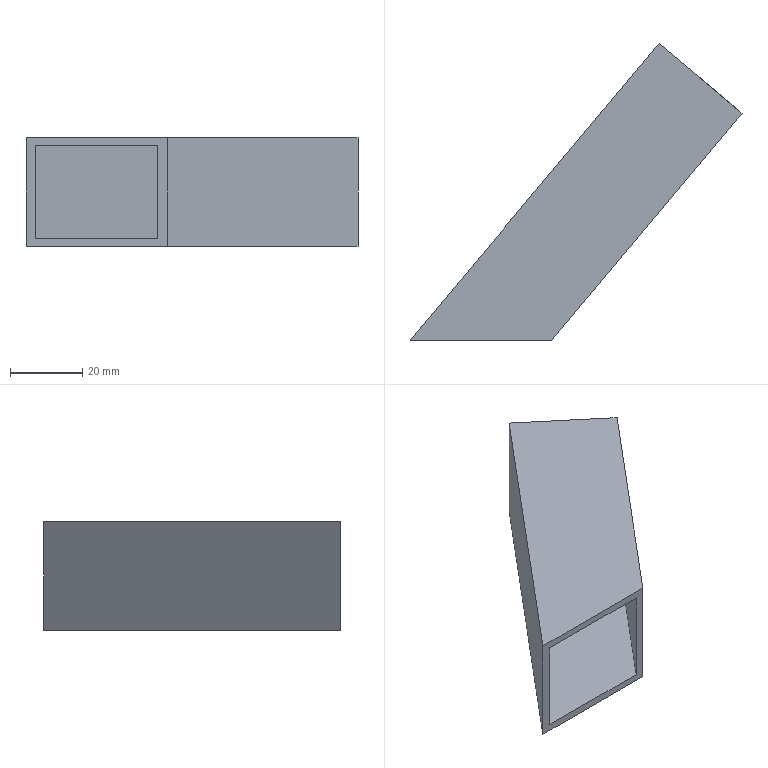Part | NX | features solid 2 | 1 solid | 10 faces | box 91.95 x 82.194 x 30 mm | volume 21215 mm3 | plane 10
STEP:
#1=CARTESIAN_POINT('',(566.959,407.194,-45.));
#2=VERTEX_POINT('',#1);
#3=CARTESIAN_POINT('',(589.941,387.91,-45.));
#4=VERTEX_POINT('',#3);
#5=CARTESIAN_POINT('',(1441.684,-326.787,-45.));
#6=DIRECTION('',(-0.766,0.6428,0.));
#7=VECTOR('',#6,1000.);
#8=LINE('',#5,#7);
#9=EDGE_CURVE('',#2,#4,#8,.F.);
#10=ORIENTED_EDGE('',*,*,#9,.T.);
#11=CARTESIAN_POINT('',(589.941,387.91,-75.));
#12=VERTEX_POINT('',#11);
#13=CARTESIAN_POINT('',(589.941,387.91,-75.));
#14=DIRECTION('',(0.,0.,1.));
#15=VECTOR('',#14,1000.);
#16=LINE('',#13,#15);
#17=EDGE_CURVE('',#12,#4,#16,.T.);
#18=ORIENTED_EDGE('',*,*,#17,.F.);
#19=CARTESIAN_POINT('',(566.959,407.194,-75.));
#20=VERTEX_POINT('',#19);
#21=CARTESIAN_POINT('',(1441.684,-326.787,-75.));
#22=DIRECTION('',(-0.766,0.6428,0.));
#23=VECTOR('',#22,1000.);
#24=LINE('',#21,#23);
#25=EDGE_CURVE('',#20,#12,#24,.F.);
#26=ORIENTED_EDGE('',*,*,#25,.F.);
#27=CARTESIAN_POINT('',(566.959,407.194,-75.));
#28=DIRECTION('',(0.,0.,1.));
#29=VECTOR('',#28,1000.);
#30=LINE('',#27,#29);
#31=EDGE_CURVE('',#20,#2,#30,.T.);
#32=ORIENTED_EDGE('',*,*,#31,.T.);
#33=EDGE_LOOP('',(#10,#18,#26,#32));
#34=FACE_BOUND('',#33,.T.);
#35=CARTESIAN_POINT('',(568.492,405.908,-47.));
#36=VERTEX_POINT('',#35);
#37=CARTESIAN_POINT('',(588.409,389.196,-47.));
#38=VERTEX_POINT('',#37);
#39=CARTESIAN_POINT('',(1441.684,-326.787,-47.));
#40=DIRECTION('',(0.766,-0.6428,0.));
#41=VECTOR('',#40,1000.);
#42=LINE('',#39,#41);
#43=EDGE_CURVE('',#36,#38,#42,.T.);
#44=ORIENTED_EDGE('',*,*,#43,.F.);
#45=CARTESIAN_POINT('',(568.492,405.908,-73.));
#46=VERTEX_POINT('',#45);
#47=CARTESIAN_POINT('',(568.492,405.908,-75.));
#48=DIRECTION('',(0.,0.,1.));
#49=VECTOR('',#48,1000.);
#50=LINE('',#47,#49);
#51=EDGE_CURVE('',#46,#36,#50,.T.);
#52=ORIENTED_EDGE('',*,*,#51,.F.);
#53=CARTESIAN_POINT('',(588.409,389.196,-73.));
#54=VERTEX_POINT('',#53);
#55=CARTESIAN_POINT('',(1441.684,-326.787,-73.));
#56=DIRECTION('',(0.766,-0.6428,0.));
#57=VECTOR('',#56,1000.);
#58=LINE('',#55,#57);
#59=EDGE_CURVE('',#46,#54,#58,.T.);
#60=ORIENTED_EDGE('',*,*,#59,.T.);
#61=CARTESIAN_POINT('',(588.409,389.196,-75.));
#62=DIRECTION('',(0.,0.,1.));
#63=VECTOR('',#62,1000.);
#64=LINE('',#61,#63);
#65=EDGE_CURVE('',#54,#38,#64,.T.);
#66=ORIENTED_EDGE('',*,*,#65,.T.);
#67=EDGE_LOOP('',(#44,#52,#60,#66));
#68=FACE_BOUND('',#67,.T.);
#69=CARTESIAN_POINT('',(1441.684,-326.787,-75.));
#70=DIRECTION('',(-0.6428,-0.766,0.));
#71=DIRECTION('',(0.766,-0.6428,0.));
#72=AXIS2_PLACEMENT_3D('',#69,#70,#71);
#73=PLANE('',#72);
#74=ADVANCED_FACE('',(#34,#68),#73,.F.);
#75=CARTESIAN_POINT('',(497.991,325.,-45.));
#76=VERTEX_POINT('',#75);
#77=CARTESIAN_POINT('',(537.153,325.,-45.));
#78=VERTEX_POINT('',#77);
#79=CARTESIAN_POINT('',(25.,325.,-45.));
#80=DIRECTION('',(-1.,0.,0.));
#81=VECTOR('',#80,1000.);
#82=LINE('',#79,#81);
#83=EDGE_CURVE('',#76,#78,#82,.F.);
#84=ORIENTED_EDGE('',*,*,#83,.F.);
#85=CARTESIAN_POINT('',(497.991,325.,-75.));
#86=VERTEX_POINT('',#85);
#87=CARTESIAN_POINT('',(497.991,325.,-75.));
#88=DIRECTION('',(0.,0.,1.));
#89=VECTOR('',#88,1000.);
#90=LINE('',#87,#89);
#91=EDGE_CURVE('',#86,#76,#90,.T.);
#92=ORIENTED_EDGE('',*,*,#91,.F.);
#93=CARTESIAN_POINT('',(537.153,325.,-75.));
#94=VERTEX_POINT('',#93);
#95=CARTESIAN_POINT('',(25.,325.,-75.));
#96=DIRECTION('',(-1.,0.,0.));
#97=VECTOR('',#96,1000.);
#98=LINE('',#95,#97);
#99=EDGE_CURVE('',#86,#94,#98,.F.);
#100=ORIENTED_EDGE('',*,*,#99,.T.);
#101=CARTESIAN_POINT('',(537.153,325.,-75.));
#102=DIRECTION('',(0.,0.,1.));
#103=VECTOR('',#102,1000.);
#104=LINE('',#101,#103);
#105=EDGE_CURVE('',#94,#78,#104,.T.);
#106=ORIENTED_EDGE('',*,*,#105,.T.);
#107=EDGE_LOOP('',(#84,#92,#100,#106));
#108=FACE_BOUND('',#107,.T.);
#109=CARTESIAN_POINT('',(500.602,325.,-73.));
#110=VERTEX_POINT('',#109);
#111=CARTESIAN_POINT('',(500.602,325.,-47.));
#112=VERTEX_POINT('',#111);
#113=CARTESIAN_POINT('',(500.602,325.,-75.));
#114=DIRECTION('',(0.,0.,1.));
#115=VECTOR('',#114,1000.);
#116=LINE('',#113,#115);
#117=EDGE_CURVE('',#110,#112,#116,.T.);
#118=ORIENTED_EDGE('',*,*,#117,.T.);
#119=CARTESIAN_POINT('',(534.542,325.,-47.));
#120=VERTEX_POINT('',#119);
#121=CARTESIAN_POINT('',(25.,325.,-47.));
#122=DIRECTION('',(-1.,0.,0.));
#123=VECTOR('',#122,1000.);
#124=LINE('',#121,#123);
#125=EDGE_CURVE('',#112,#120,#124,.F.);
#126=ORIENTED_EDGE('',*,*,#125,.T.);
#127=CARTESIAN_POINT('',(534.542,325.,-73.));
#128=VERTEX_POINT('',#127);
#129=CARTESIAN_POINT('',(534.542,325.,-75.));
#130=DIRECTION('',(0.,0.,1.));
#131=VECTOR('',#130,1000.);
#132=LINE('',#129,#131);
#133=EDGE_CURVE('',#128,#120,#132,.T.);
#134=ORIENTED_EDGE('',*,*,#133,.F.);
#135=CARTESIAN_POINT('',(25.,325.,-73.));
#136=DIRECTION('',(-1.,0.,0.));
#137=VECTOR('',#136,1000.);
#138=LINE('',#135,#137);
#139=EDGE_CURVE('',#110,#128,#138,.F.);
#140=ORIENTED_EDGE('',*,*,#139,.F.);
#141=EDGE_LOOP('',(#118,#126,#134,#140));
#142=FACE_BOUND('',#141,.T.);
#143=CARTESIAN_POINT('',(25.,325.,-75.));
#144=DIRECTION('',(0.,-1.,0.));
#145=DIRECTION('',(1.,0.,0.));
#146=AXIS2_PLACEMENT_3D('',#143,#144,#145);
#147=PLANE('',#146);
#148=ADVANCED_FACE('',(#108,#142),#147,.T.);
#149=CARTESIAN_POINT('',(525.178,357.401,-45.));
#150=DIRECTION('',(-0.6428,-0.766,0.));
#151=VECTOR('',#150,1000.);
#152=LINE('',#149,#151);
#153=EDGE_CURVE('',#76,#2,#152,.F.);
#154=ORIENTED_EDGE('',*,*,#153,.T.);
#155=ORIENTED_EDGE('',*,*,#31,.F.);
#156=CARTESIAN_POINT('',(525.178,357.401,-75.));
#157=DIRECTION('',(-0.6428,-0.766,0.));
#158=VECTOR('',#157,1000.);
#159=LINE('',#156,#158);
#160=EDGE_CURVE('',#86,#20,#159,.F.);
#161=ORIENTED_EDGE('',*,*,#160,.F.);
#162=ORIENTED_EDGE('',*,*,#91,.T.);
#163=EDGE_LOOP('',(#154,#155,#161,#162));
#164=FACE_BOUND('',#163,.T.);
#165=CARTESIAN_POINT('',(525.178,357.401,-75.));
#166=DIRECTION('',(0.766,-0.6428,0.));
#167=DIRECTION('',(0.6428,0.766,0.));
#168=AXIS2_PLACEMENT_3D('',#165,#166,#167);
#169=PLANE('',#168);
#170=ADVANCED_FACE('',(#164),#169,.F.);
#171=CARTESIAN_POINT('',(548.16,338.117,-45.));
#172=DIRECTION('',(-0.6428,-0.766,0.));
#173=VECTOR('',#172,1000.);
#174=LINE('',#171,#173);
#175=EDGE_CURVE('',#78,#4,#174,.F.);
#176=ORIENTED_EDGE('',*,*,#175,.F.);
#177=ORIENTED_EDGE('',*,*,#105,.F.);
#178=CARTESIAN_POINT('',(548.16,338.117,-75.));
#179=DIRECTION('',(-0.6428,-0.766,0.));
#180=VECTOR('',#179,1000.);
#181=LINE('',#178,#180);
#182=EDGE_CURVE('',#94,#12,#181,.F.);
#183=ORIENTED_EDGE('',*,*,#182,.T.);
#184=ORIENTED_EDGE('',*,*,#17,.T.);
#185=EDGE_LOOP('',(#176,#177,#183,#184));
#186=FACE_BOUND('',#185,.T.);
#187=CARTESIAN_POINT('',(548.16,338.117,-75.));
#188=DIRECTION('',(0.766,-0.6428,0.));
#189=DIRECTION('',(0.6428,0.766,0.));
#190=AXIS2_PLACEMENT_3D('',#187,#188,#189);
#191=PLANE('',#190);
#192=ADVANCED_FACE('',(#186),#191,.T.);
#193=ORIENTED_EDGE('',*,*,#99,.F.);
#194=ORIENTED_EDGE('',*,*,#160,.T.);
#195=ORIENTED_EDGE('',*,*,#25,.T.);
#196=ORIENTED_EDGE('',*,*,#182,.F.);
#197=EDGE_LOOP('',(#193,#194,#195,#196));
#198=FACE_BOUND('',#197,.T.);
#199=CARTESIAN_POINT('',(1076.581,-761.9,-75.));
#200=DIRECTION('',(0.,0.,1.));
#201=DIRECTION('',(1.,0.,0.));
#202=AXIS2_PLACEMENT_3D('',#199,#200,#201);
#203=PLANE('',#202);
#204=ADVANCED_FACE('',(#198),#203,.F.);
#205=ORIENTED_EDGE('',*,*,#83,.T.);
#206=ORIENTED_EDGE('',*,*,#175,.T.);
#207=ORIENTED_EDGE('',*,*,#9,.F.);
#208=ORIENTED_EDGE('',*,*,#153,.F.);
#209=EDGE_LOOP('',(#205,#206,#207,#208));
#210=FACE_BOUND('',#209,.T.);
#211=CARTESIAN_POINT('',(1076.581,-761.9,-45.));
#212=DIRECTION('',(0.,0.,1.));
#213=DIRECTION('',(1.,0.,0.));
#214=AXIS2_PLACEMENT_3D('',#211,#212,#213);
#215=PLANE('',#214);
#216=ADVANCED_FACE('',(#210),#215,.T.);
#217=CARTESIAN_POINT('',(526.71,356.115,-47.));
#218=DIRECTION('',(-0.6428,-0.766,0.));
#219=VECTOR('',#218,1000.);
#220=LINE('',#217,#219);
#221=EDGE_CURVE('',#112,#36,#220,.F.);
#222=ORIENTED_EDGE('',*,*,#221,.F.);
#223=ORIENTED_EDGE('',*,*,#117,.F.);
#224=CARTESIAN_POINT('',(526.71,356.115,-73.));
#225=DIRECTION('',(-0.6428,-0.766,0.));
#226=VECTOR('',#225,1000.);
#227=LINE('',#224,#226);
#228=EDGE_CURVE('',#110,#46,#227,.F.);
#229=ORIENTED_EDGE('',*,*,#228,.T.);
#230=ORIENTED_EDGE('',*,*,#51,.T.);
#231=EDGE_LOOP('',(#222,#223,#229,#230));
#232=FACE_BOUND('',#231,.T.);
#233=CARTESIAN_POINT('',(526.71,356.115,-75.));
#234=DIRECTION('',(0.766,-0.6428,0.));
#235=DIRECTION('',(0.6428,0.766,0.));
#236=AXIS2_PLACEMENT_3D('',#233,#234,#235);
#237=PLANE('',#236);
#238=ADVANCED_FACE('',(#232),#237,.T.);
#239=CARTESIAN_POINT('',(546.628,339.403,-47.));
#240=DIRECTION('',(-0.6428,-0.766,0.));
#241=VECTOR('',#240,1000.);
#242=LINE('',#239,#241);
#243=EDGE_CURVE('',#120,#38,#242,.F.);
#244=ORIENTED_EDGE('',*,*,#243,.T.);
#245=ORIENTED_EDGE('',*,*,#65,.F.);
#246=CARTESIAN_POINT('',(546.628,339.403,-73.));
#247=DIRECTION('',(-0.6428,-0.766,0.));
#248=VECTOR('',#247,1000.);
#249=LINE('',#246,#248);
#250=EDGE_CURVE('',#128,#54,#249,.F.);
#251=ORIENTED_EDGE('',*,*,#250,.F.);
#252=ORIENTED_EDGE('',*,*,#133,.T.);
#253=EDGE_LOOP('',(#244,#245,#251,#252));
#254=FACE_BOUND('',#253,.T.);
#255=CARTESIAN_POINT('',(546.628,339.403,-75.));
#256=DIRECTION('',(0.766,-0.6428,0.));
#257=DIRECTION('',(0.6428,0.766,0.));
#258=AXIS2_PLACEMENT_3D('',#255,#256,#257);
#259=PLANE('',#258);
#260=ADVANCED_FACE('',(#254),#259,.F.);
#261=ORIENTED_EDGE('',*,*,#139,.T.);
#262=ORIENTED_EDGE('',*,*,#250,.T.);
#263=ORIENTED_EDGE('',*,*,#59,.F.);
#264=ORIENTED_EDGE('',*,*,#228,.F.);
#265=EDGE_LOOP('',(#261,#262,#263,#264));
#266=FACE_BOUND('',#265,.T.);
#267=CARTESIAN_POINT('',(1076.581,-761.9,-73.));
#268=DIRECTION('',(0.,0.,1.));
#269=DIRECTION('',(1.,0.,0.));
#270=AXIS2_PLACEMENT_3D('',#267,#268,#269);
#271=PLANE('',#270);
#272=ADVANCED_FACE('',(#266),#271,.T.);
#273=ORIENTED_EDGE('',*,*,#125,.F.);
#274=ORIENTED_EDGE('',*,*,#221,.T.);
#275=ORIENTED_EDGE('',*,*,#43,.T.);
#276=ORIENTED_EDGE('',*,*,#243,.F.);
#277=EDGE_LOOP('',(#273,#274,#275,#276));
#278=FACE_BOUND('',#277,.T.);
#279=CARTESIAN_POINT('',(1076.581,-761.9,-47.));
#280=DIRECTION('',(0.,0.,1.));
#281=DIRECTION('',(1.,0.,0.));
#282=AXIS2_PLACEMENT_3D('',#279,#280,#281);
#283=PLANE('',#282);
#284=ADVANCED_FACE('',(#278),#283,.F.);
#285=CLOSED_SHELL('',(#74,#148,#170,#192,#204,#216,#238,#260,#272,#284));
#286=MANIFOLD_SOLID_BREP('',#285);
#287=(LENGTH_UNIT()NAMED_UNIT(*)SI_UNIT(.MILLI.,.METRE.));
#288=UNCERTAINTY_MEASURE_WITH_UNIT(LENGTH_MEASURE(0.00001),#287,'','');
#289=(NAMED_UNIT(*)PLANE_ANGLE_UNIT()SI_UNIT($,.RADIAN.));
#290=(NAMED_UNIT(*)SI_UNIT($,.STERADIAN.)SOLID_ANGLE_UNIT());
#291=(GEOMETRIC_REPRESENTATION_CONTEXT(3)GLOBAL_UNCERTAINTY_ASSIGNED_CONTEXT((#288))GLOBAL_UNIT_ASSIGNED_CONTEXT((#287,#289,#290))REPRESENTATION_CONTEXT('',''));
#292=ADVANCED_BREP_SHAPE_REPRESENTATION('',(#286),#291);